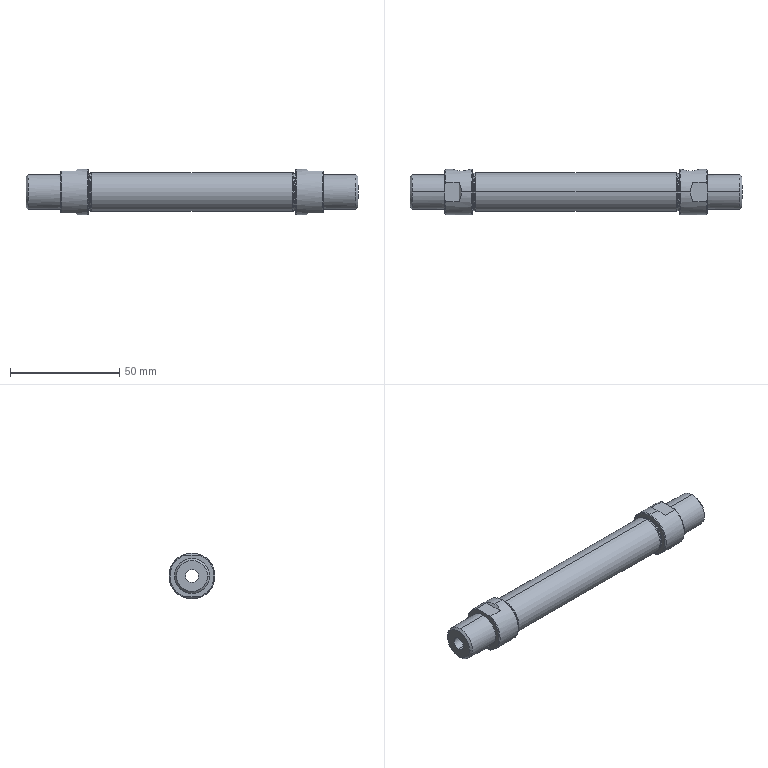Part | STEP file | _16MAD60Body | 1 solid | 72 faces | box 152 x 21 x 21 mm | volume 19082 mm3 | cylinder 24 | plane 20 | spline 16 | cone 12 | commonest cylinder face diameters 16 x6 4.134 x4 6 x4 8.5 x4 21 x4 17.4 x2